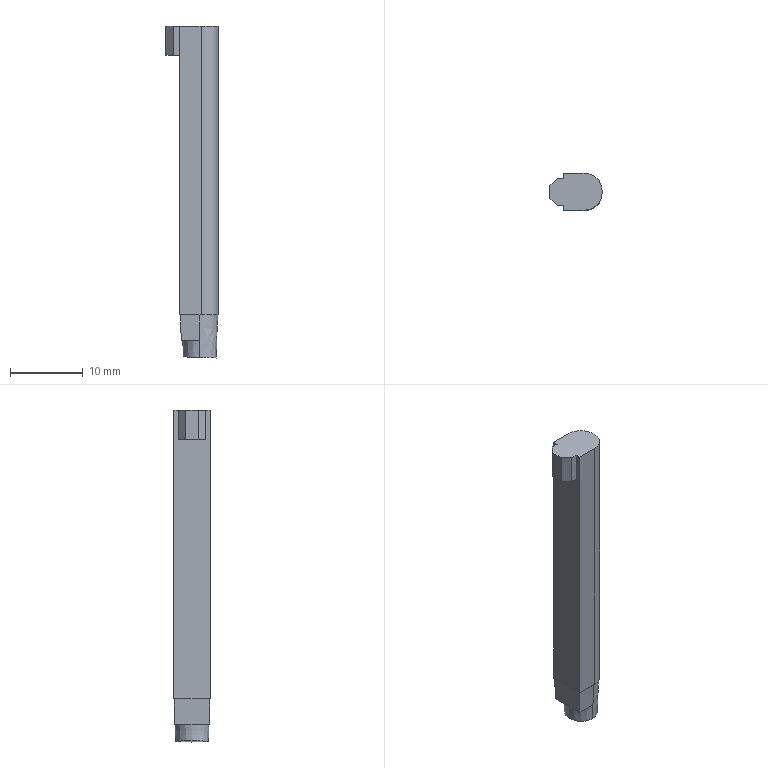Part | Creo | 1 solid | 21 faces | box 7.184 x 5.033 x 45.741 mm | volume 1104 mm3 | plane 17 | cylinder 2 | spline 2 | commonest cylinder face diameters 4.7 x2
STEP:
#1=CARTESIAN_POINT('',(0.,0.,0.));
#2=DIRECTION('',(0.,0.,1.));
#3=DIRECTION('',(1.,0.,0.));
#4=AXIS2_PLACEMENT_3D('',#1,#2,#3);
#5=CARTESIAN_POINT('',(-43.549,78.476,85.91));
#6=VERTEX_POINT('',#5);
#7=CARTESIAN_POINT('',(-43.549,78.476,46.111));
#8=VERTEX_POINT('',#7);
#9=CARTESIAN_POINT('',(-43.549,78.476,85.91));
#10=DIRECTION('',(0.,0.,-1.));
#11=VECTOR('',#10,39.799);
#12=LINE('',#9,#11);
#13=EDGE_CURVE('',#6,#8,#12,.T.);
#14=ORIENTED_EDGE('',*,*,#13,.F.);
#15=CARTESIAN_POINT('',(-40.614,78.476,85.91));
#16=VERTEX_POINT('',#15);
#17=CARTESIAN_POINT('',(-43.549,78.476,85.91));
#18=DIRECTION('',(1.,0.,0.));
#19=VECTOR('',#18,2.934);
#20=LINE('',#17,#19);
#21=EDGE_CURVE('',#6,#16,#20,.T.);
#22=ORIENTED_EDGE('',*,*,#21,.T.);
#23=CARTESIAN_POINT('',(-40.614,78.476,46.111));
#24=VERTEX_POINT('',#23);
#25=CARTESIAN_POINT('',(-40.614,78.476,85.91));
#26=DIRECTION('',(0.,0.,-1.));
#27=VECTOR('',#26,39.799);
#28=LINE('',#25,#27);
#29=EDGE_CURVE('',#16,#24,#28,.T.);
#30=ORIENTED_EDGE('',*,*,#29,.T.);
#31=CARTESIAN_POINT('',(-40.614,78.476,46.111));
#32=DIRECTION('',(-1.,0.,0.));
#33=VECTOR('',#32,2.934);
#34=LINE('',#31,#33);
#35=EDGE_CURVE('',#24,#8,#34,.T.);
#36=ORIENTED_EDGE('',*,*,#35,.T.);
#37=EDGE_LOOP('',(#14,#22,#30,#36));
#38=FACE_OUTER_BOUND('',#37,.F.);
#39=CARTESIAN_POINT('',(-40.806,78.476,6.695));
#40=DIRECTION('',(0.,-1.,0.));
#41=DIRECTION('',(0.,0.,-1.));
#42=AXIS2_PLACEMENT_3D('',#39,#40,#41);
#43=PLANE('',#42);
#44=ADVANCED_FACE('',(#38),#43,.T.);
#45=CARTESIAN_POINT('',(-43.549,83.509,85.91));
#46=VERTEX_POINT('',#45);
#47=CARTESIAN_POINT('',(-43.549,83.509,46.111));
#48=VERTEX_POINT('',#47);
#49=CARTESIAN_POINT('',(-43.549,83.509,85.91));
#50=DIRECTION('',(0.,0.,-1.));
#51=VECTOR('',#50,39.799);
#52=LINE('',#49,#51);
#53=EDGE_CURVE('',#46,#48,#52,.T.);
#54=ORIENTED_EDGE('',*,*,#53,.F.);
#55=CARTESIAN_POINT('',(-43.549,82.859,85.91));
#56=VERTEX_POINT('',#55);
#57=CARTESIAN_POINT('',(-43.549,83.509,85.91));
#58=DIRECTION('',(0.,-1.,0.));
#59=VECTOR('',#58,0.65);
#60=LINE('',#57,#59);
#61=EDGE_CURVE('',#46,#56,#60,.T.);
#62=ORIENTED_EDGE('',*,*,#61,.T.);
#63=CARTESIAN_POINT('',(-43.549,82.859,81.91));
#64=VERTEX_POINT('',#63);
#65=CARTESIAN_POINT('',(-43.549,82.859,81.91));
#66=DIRECTION('',(0.,0.,1.));
#67=VECTOR('',#66,4.);
#68=LINE('',#65,#67);
#69=EDGE_CURVE('',#64,#56,#68,.T.);
#70=ORIENTED_EDGE('',*,*,#69,.F.);
#71=CARTESIAN_POINT('',(-43.549,79.126,81.91));
#72=VERTEX_POINT('',#71);
#73=CARTESIAN_POINT('',(-43.549,79.126,81.91));
#74=DIRECTION('',(0.,1.,0.));
#75=VECTOR('',#74,3.733);
#76=LINE('',#73,#75);
#77=EDGE_CURVE('',#72,#64,#76,.T.);
#78=ORIENTED_EDGE('',*,*,#77,.F.);
#79=CARTESIAN_POINT('',(-43.549,79.126,85.91));
#80=VERTEX_POINT('',#79);
#81=CARTESIAN_POINT('',(-43.549,79.126,85.91));
#82=DIRECTION('',(0.,0.,-1.));
#83=VECTOR('',#82,4.);
#84=LINE('',#81,#83);
#85=EDGE_CURVE('',#80,#72,#84,.T.);
#86=ORIENTED_EDGE('',*,*,#85,.F.);
#87=CARTESIAN_POINT('',(-43.549,79.126,85.91));
#88=DIRECTION('',(0.,-1.,0.));
#89=VECTOR('',#88,0.65);
#90=LINE('',#87,#89);
#91=EDGE_CURVE('',#80,#6,#90,.T.);
#92=ORIENTED_EDGE('',*,*,#91,.T.);
#93=ORIENTED_EDGE('',*,*,#13,.T.);
#94=CARTESIAN_POINT('',(-43.549,78.476,46.111));
#95=DIRECTION('',(0.,1.,0.));
#96=VECTOR('',#95,5.033);
#97=LINE('',#94,#96);
#98=EDGE_CURVE('',#8,#48,#97,.T.);
#99=ORIENTED_EDGE('',*,*,#98,.T.);
#100=EDGE_LOOP('',(#54,#62,#70,#78,#86,#92,#93,#99));
#101=FACE_OUTER_BOUND('',#100,.F.);
#102=CARTESIAN_POINT('',(-43.549,80.993,6.695));
#103=DIRECTION('',(-1.,0.,0.));
#104=DIRECTION('',(0.,0.,1.));
#105=AXIS2_PLACEMENT_3D('',#102,#103,#104);
#106=PLANE('',#105);
#107=ADVANCED_FACE('',(#101),#106,.T.);
#108=CARTESIAN_POINT('',(-40.614,83.509,46.111));
#109=VERTEX_POINT('',#108);
#110=CARTESIAN_POINT('',(-40.614,83.509,85.91));
#111=VERTEX_POINT('',#110);
#112=CARTESIAN_POINT('',(-40.614,83.509,46.111));
#113=DIRECTION('',(0.,0.,1.));
#114=VECTOR('',#113,39.799);
#115=LINE('',#112,#114);
#116=EDGE_CURVE('',#109,#111,#115,.T.);
#117=ORIENTED_EDGE('',*,*,#116,.T.);
#118=CARTESIAN_POINT('',(-40.614,83.509,85.91));
#119=DIRECTION('',(-1.,0.,0.));
#120=VECTOR('',#119,2.934);
#121=LINE('',#118,#120);
#122=EDGE_CURVE('',#111,#46,#121,.T.);
#123=ORIENTED_EDGE('',*,*,#122,.T.);
#124=ORIENTED_EDGE('',*,*,#53,.T.);
#125=CARTESIAN_POINT('',(-43.549,83.509,46.111));
#126=DIRECTION('',(1.,0.,0.));
#127=VECTOR('',#126,2.934);
#128=LINE('',#125,#127);
#129=EDGE_CURVE('',#48,#109,#128,.T.);
#130=ORIENTED_EDGE('',*,*,#129,.T.);
#131=EDGE_LOOP('',(#117,#123,#124,#130));
#132=FACE_OUTER_BOUND('',#131,.F.);
#133=CARTESIAN_POINT('',(-40.806,83.509,6.695));
#134=DIRECTION('',(0.,1.,0.));
#135=DIRECTION('',(0.,0.,1.));
#136=AXIS2_PLACEMENT_3D('',#133,#134,#135);
#137=PLANE('',#136);
#138=ADVANCED_FACE('',(#132),#137,.T.);
#139=CARTESIAN_POINT('',(-38.264,81.159,85.91));
#140=VERTEX_POINT('',#139);
#141=CARTESIAN_POINT('',(-38.264,81.159,46.111));
#142=VERTEX_POINT('',#141);
#143=CARTESIAN_POINT('',(-38.264,81.159,85.91));
#144=DIRECTION('',(0.,0.,-1.));
#145=VECTOR('',#144,39.799);
#146=LINE('',#143,#145);
#147=EDGE_CURVE('',#140,#142,#146,.T.);
#148=ORIENTED_EDGE('',*,*,#147,.F.);
#149=CARTESIAN_POINT('',(-40.614,81.159,85.91));
#150=DIRECTION('',(0.,0.,1.));
#151=DIRECTION('',(1.,0.,0.));
#152=AXIS2_PLACEMENT_3D('',#149,#150,#151);
#153=CIRCLE('',#152,2.35);
#154=EDGE_CURVE('',#140,#111,#153,.T.);
#155=ORIENTED_EDGE('',*,*,#154,.T.);
#156=ORIENTED_EDGE('',*,*,#116,.F.);
#157=CARTESIAN_POINT('',(-40.614,81.159,46.111));
#158=DIRECTION('',(0.,0.,-1.));
#159=DIRECTION('',(0.,1.,0.));
#160=AXIS2_PLACEMENT_3D('',#157,#158,#159);
#161=CIRCLE('',#160,2.35);
#162=EDGE_CURVE('',#109,#142,#161,.T.);
#163=ORIENTED_EDGE('',*,*,#162,.T.);
#164=EDGE_LOOP('',(#148,#155,#156,#163));
#165=FACE_OUTER_BOUND('',#164,.F.);
#166=CARTESIAN_POINT('',(-40.614,81.159,6.695));
#167=DIRECTION('',(0.,0.,1.));
#168=DIRECTION('',(1.,0.,0.));
#169=AXIS2_PLACEMENT_3D('',#166,#167,#168);
#170=CYLINDRICAL_SURFACE('',#169,2.35);
#171=ADVANCED_FACE('',(#165),#170,.T.);
#172=CARTESIAN_POINT('',(-38.264,80.826,46.111));
#173=VERTEX_POINT('',#172);
#174=CARTESIAN_POINT('',(-38.264,80.826,85.91));
#175=VERTEX_POINT('',#174);
#176=CARTESIAN_POINT('',(-38.264,80.826,46.111));
#177=DIRECTION('',(0.,0.,1.));
#178=VECTOR('',#177,39.799);
#179=LINE('',#176,#178);
#180=EDGE_CURVE('',#173,#175,#179,.T.);
#181=ORIENTED_EDGE('',*,*,#180,.T.);
#182=CARTESIAN_POINT('',(-38.264,80.826,85.91));
#183=DIRECTION('',(0.,1.,0.));
#184=VECTOR('',#183,0.333);
#185=LINE('',#182,#184);
#186=EDGE_CURVE('',#175,#140,#185,.T.);
#187=ORIENTED_EDGE('',*,*,#186,.T.);
#188=ORIENTED_EDGE('',*,*,#147,.T.);
#189=CARTESIAN_POINT('',(-38.264,81.159,46.111));
#190=DIRECTION('',(0.,-1.,0.));
#191=VECTOR('',#190,0.333);
#192=LINE('',#189,#191);
#193=EDGE_CURVE('',#142,#173,#192,.T.);
#194=ORIENTED_EDGE('',*,*,#193,.T.);
#195=EDGE_LOOP('',(#181,#187,#188,#194));
#196=FACE_OUTER_BOUND('',#195,.F.);
#197=CARTESIAN_POINT('',(-38.264,80.993,6.695));
#198=DIRECTION('',(1.,0.,0.));
#199=DIRECTION('',(0.,0.,-1.));
#200=AXIS2_PLACEMENT_3D('',#197,#198,#199);
#201=PLANE('',#200);
#202=ADVANCED_FACE('',(#196),#201,.T.);
#203=ORIENTED_EDGE('',*,*,#29,.F.);
#204=CARTESIAN_POINT('',(-40.614,80.826,85.91));
#205=DIRECTION('',(0.,0.,1.));
#206=DIRECTION('',(0.,-1.,0.));
#207=AXIS2_PLACEMENT_3D('',#204,#205,#206);
#208=CIRCLE('',#207,2.35);
#209=EDGE_CURVE('',#16,#175,#208,.T.);
#210=ORIENTED_EDGE('',*,*,#209,.T.);
#211=ORIENTED_EDGE('',*,*,#180,.F.);
#212=CARTESIAN_POINT('',(-40.614,80.826,46.111));
#213=DIRECTION('',(0.,0.,-1.));
#214=DIRECTION('',(1.,0.,0.));
#215=AXIS2_PLACEMENT_3D('',#212,#213,#214);
#216=CIRCLE('',#215,2.35);
#217=EDGE_CURVE('',#173,#24,#216,.T.);
#218=ORIENTED_EDGE('',*,*,#217,.T.);
#219=EDGE_LOOP('',(#203,#210,#211,#218));
#220=FACE_OUTER_BOUND('',#219,.F.);
#221=CARTESIAN_POINT('',(-40.614,80.826,6.695));
#222=DIRECTION('',(0.,0.,1.));
#223=DIRECTION('',(1.,0.,0.));
#224=AXIS2_PLACEMENT_3D('',#221,#222,#223);
#225=CYLINDRICAL_SURFACE('',#224,2.35);
#226=ADVANCED_FACE('',(#220),#225,.T.);
#227=CARTESIAN_POINT('',(-45.449,81.859,85.91));
#228=VERTEX_POINT('',#227);
#229=CARTESIAN_POINT('',(-45.449,80.126,85.91));
#230=VERTEX_POINT('',#229);
#231=CARTESIAN_POINT('',(-45.449,81.859,85.91));
#232=DIRECTION('',(0.,-1.,0.));
#233=VECTOR('',#232,1.733);
#234=LINE('',#231,#233);
#235=EDGE_CURVE('',#228,#230,#234,.T.);
#236=ORIENTED_EDGE('',*,*,#235,.F.);
#237=CARTESIAN_POINT('',(-44.449,82.859,85.91));
#238=VERTEX_POINT('',#237);
#239=CARTESIAN_POINT('',(-44.449,82.859,85.91));
#240=DIRECTION('',(-0.7071,-0.7071,0.));
#241=VECTOR('',#240,1.414);
#242=LINE('',#239,#241);
#243=EDGE_CURVE('',#238,#228,#242,.T.);
#244=ORIENTED_EDGE('',*,*,#243,.F.);
#245=CARTESIAN_POINT('',(-43.549,82.859,85.91));
#246=DIRECTION('',(-1.,0.,0.));
#247=VECTOR('',#246,0.9);
#248=LINE('',#245,#247);
#249=EDGE_CURVE('',#56,#238,#248,.T.);
#250=ORIENTED_EDGE('',*,*,#249,.F.);
#251=ORIENTED_EDGE('',*,*,#61,.F.);
#252=ORIENTED_EDGE('',*,*,#122,.F.);
#253=ORIENTED_EDGE('',*,*,#154,.F.);
#254=ORIENTED_EDGE('',*,*,#186,.F.);
#255=ORIENTED_EDGE('',*,*,#209,.F.);
#256=ORIENTED_EDGE('',*,*,#21,.F.);
#257=ORIENTED_EDGE('',*,*,#91,.F.);
#258=CARTESIAN_POINT('',(-44.449,79.126,85.91));
#259=VERTEX_POINT('',#258);
#260=CARTESIAN_POINT('',(-44.449,79.126,85.91));
#261=DIRECTION('',(1.,0.,0.));
#262=VECTOR('',#261,0.9);
#263=LINE('',#260,#262);
#264=EDGE_CURVE('',#259,#80,#263,.T.);
#265=ORIENTED_EDGE('',*,*,#264,.F.);
#266=CARTESIAN_POINT('',(-45.449,80.126,85.91));
#267=DIRECTION('',(0.7071,-0.7071,0.));
#268=VECTOR('',#267,1.414);
#269=LINE('',#266,#268);
#270=EDGE_CURVE('',#230,#259,#269,.T.);
#271=ORIENTED_EDGE('',*,*,#270,.F.);
#272=EDGE_LOOP('',(#236,#244,#250,#251,#252,#253,#254,#255,#256,#257,#265,#271));
#273=FACE_OUTER_BOUND('',#272,.F.);
#274=CARTESIAN_POINT('',(62.144,-0.4125,85.91));
#275=DIRECTION('',(0.,0.,1.));
#276=DIRECTION('',(0.,1.,0.));
#277=AXIS2_PLACEMENT_3D('',#274,#275,#276);
#278=PLANE('',#277);
#279=ADVANCED_FACE('',(#273),#278,.T.);
#280=CARTESIAN_POINT('',(-45.449,80.126,81.91));
#281=VERTEX_POINT('',#280);
#282=CARTESIAN_POINT('',(-45.449,81.859,81.91));
#283=VERTEX_POINT('',#282);
#284=CARTESIAN_POINT('',(-45.449,80.126,81.91));
#285=DIRECTION('',(0.,1.,0.));
#286=VECTOR('',#285,1.733);
#287=LINE('',#284,#286);
#288=EDGE_CURVE('',#281,#283,#287,.T.);
#289=ORIENTED_EDGE('',*,*,#288,.T.);
#290=CARTESIAN_POINT('',(-45.449,81.859,81.91));
#291=DIRECTION('',(0.,0.,1.));
#292=VECTOR('',#291,4.);
#293=LINE('',#290,#292);
#294=EDGE_CURVE('',#283,#228,#293,.T.);
#295=ORIENTED_EDGE('',*,*,#294,.T.);
#296=ORIENTED_EDGE('',*,*,#235,.T.);
#297=CARTESIAN_POINT('',(-45.449,80.126,85.91));
#298=DIRECTION('',(0.,0.,-1.));
#299=VECTOR('',#298,4.);
#300=LINE('',#297,#299);
#301=EDGE_CURVE('',#230,#281,#300,.T.);
#302=ORIENTED_EDGE('',*,*,#301,.T.);
#303=EDGE_LOOP('',(#289,#295,#296,#302));
#304=FACE_OUTER_BOUND('',#303,.F.);
#305=CARTESIAN_POINT('',(-45.449,80.993,81.91));
#306=DIRECTION('',(-1.,0.,0.));
#307=DIRECTION('',(0.,0.,1.));
#308=AXIS2_PLACEMENT_3D('',#305,#306,#307);
#309=PLANE('',#308);
#310=ADVANCED_FACE('',(#304),#309,.T.);
#311=CARTESIAN_POINT('',(-44.449,79.126,81.91));
#312=VERTEX_POINT('',#311);
#313=CARTESIAN_POINT('',(-43.549,79.126,81.91));
#314=DIRECTION('',(-1.,0.,0.));
#315=VECTOR('',#314,0.9);
#316=LINE('',#313,#315);
#317=EDGE_CURVE('',#72,#312,#316,.T.);
#318=ORIENTED_EDGE('',*,*,#317,.F.);
#319=ORIENTED_EDGE('',*,*,#77,.T.);
#320=CARTESIAN_POINT('',(-44.449,82.859,81.91));
#321=VERTEX_POINT('',#320);
#322=CARTESIAN_POINT('',(-44.449,82.859,81.91));
#323=DIRECTION('',(1.,0.,0.));
#324=VECTOR('',#323,0.9);
#325=LINE('',#322,#324);
#326=EDGE_CURVE('',#321,#64,#325,.T.);
#327=ORIENTED_EDGE('',*,*,#326,.F.);
#328=CARTESIAN_POINT('',(-45.449,81.859,81.91));
#329=DIRECTION('',(0.7071,0.7071,0.));
#330=VECTOR('',#329,1.414);
#331=LINE('',#328,#330);
#332=EDGE_CURVE('',#283,#321,#331,.T.);
#333=ORIENTED_EDGE('',*,*,#332,.F.);
#334=ORIENTED_EDGE('',*,*,#288,.F.);
#335=CARTESIAN_POINT('',(-44.449,79.126,81.91));
#336=DIRECTION('',(-0.7071,0.7071,0.));
#337=VECTOR('',#336,1.414);
#338=LINE('',#335,#337);
#339=EDGE_CURVE('',#312,#281,#338,.T.);
#340=ORIENTED_EDGE('',*,*,#339,.F.);
#341=EDGE_LOOP('',(#318,#319,#327,#333,#334,#340));
#342=FACE_OUTER_BOUND('',#341,.F.);
#343=CARTESIAN_POINT('',(-43.899,80.993,81.91));
#344=DIRECTION('',(0.,0.,-1.));
#345=DIRECTION('',(-1.,0.,0.));
#346=AXIS2_PLACEMENT_3D('',#343,#344,#345);
#347=PLANE('',#346);
#348=ADVANCED_FACE('',(#342),#347,.T.);
#349=ORIENTED_EDGE('',*,*,#264,.T.);
#350=ORIENTED_EDGE('',*,*,#85,.T.);
#351=ORIENTED_EDGE('',*,*,#317,.T.);
#352=CARTESIAN_POINT('',(-44.449,79.126,81.91));
#353=DIRECTION('',(0.,0.,1.));
#354=VECTOR('',#353,4.);
#355=LINE('',#352,#354);
#356=EDGE_CURVE('',#312,#259,#355,.T.);
#357=ORIENTED_EDGE('',*,*,#356,.T.);
#358=EDGE_LOOP('',(#349,#350,#351,#357));
#359=FACE_OUTER_BOUND('',#358,.F.);
#360=CARTESIAN_POINT('',(-43.899,79.126,81.91));
#361=DIRECTION('',(0.,-1.,0.));
#362=DIRECTION('',(0.,0.,-1.));
#363=AXIS2_PLACEMENT_3D('',#360,#361,#362);
#364=PLANE('',#363);
#365=ADVANCED_FACE('',(#359),#364,.T.);
#366=ORIENTED_EDGE('',*,*,#339,.T.);
#367=ORIENTED_EDGE('',*,*,#301,.F.);
#368=ORIENTED_EDGE('',*,*,#270,.T.);
#369=ORIENTED_EDGE('',*,*,#356,.F.);
#370=EDGE_LOOP('',(#366,#367,#368,#369));
#371=FACE_OUTER_BOUND('',#370,.F.);
#372=CARTESIAN_POINT('',(-45.449,80.126,81.91));
#373=DIRECTION('',(0.7071,0.7071,0.));
#374=DIRECTION('',(0.,0.,1.));
#375=AXIS2_PLACEMENT_3D('',#372,#373,#374);
#376=PLANE('',#375);
#377=ADVANCED_FACE('',(#371),#376,.F.);
#378=ORIENTED_EDGE('',*,*,#326,.T.);
#379=ORIENTED_EDGE('',*,*,#69,.T.);
#380=ORIENTED_EDGE('',*,*,#249,.T.);
#381=CARTESIAN_POINT('',(-44.449,82.859,85.91));
#382=DIRECTION('',(0.,0.,-1.));
#383=VECTOR('',#382,4.);
#384=LINE('',#381,#383);
#385=EDGE_CURVE('',#238,#321,#384,.T.);
#386=ORIENTED_EDGE('',*,*,#385,.T.);
#387=EDGE_LOOP('',(#378,#379,#380,#386));
#388=FACE_OUTER_BOUND('',#387,.F.);
#389=CARTESIAN_POINT('',(-43.899,82.859,81.91));
#390=DIRECTION('',(0.,1.,0.));
#391=DIRECTION('',(0.,0.,1.));
#392=AXIS2_PLACEMENT_3D('',#389,#390,#391);
#393=PLANE('',#392);
#394=ADVANCED_FACE('',(#388),#393,.T.);
#395=ORIENTED_EDGE('',*,*,#332,.T.);
#396=ORIENTED_EDGE('',*,*,#385,.F.);
#397=ORIENTED_EDGE('',*,*,#243,.T.);
#398=ORIENTED_EDGE('',*,*,#294,.F.);
#399=EDGE_LOOP('',(#395,#396,#397,#398));
#400=FACE_OUTER_BOUND('',#399,.F.);
#401=CARTESIAN_POINT('',(-44.449,82.859,81.91));
#402=DIRECTION('',(0.7071,-0.7071,0.));
#403=DIRECTION('',(0.,0.,1.));
#404=AXIS2_PLACEMENT_3D('',#401,#402,#403);
#405=PLANE('',#404);
#406=ADVANCED_FACE('',(#400),#405,.F.);
#407=ORIENTED_EDGE('',*,*,#217,.F.);
#408=ORIENTED_EDGE('',*,*,#193,.F.);
#409=ORIENTED_EDGE('',*,*,#162,.F.);
#410=ORIENTED_EDGE('',*,*,#129,.F.);
#411=ORIENTED_EDGE('',*,*,#98,.F.);
#412=ORIENTED_EDGE('',*,*,#35,.F.);
#413=EDGE_LOOP('',(#407,#408,#409,#410,#411,#412));
#414=FACE_OUTER_BOUND('',#413,.F.);
#415=CARTESIAN_POINT('',(-38.311,80.993,46.111));
#416=VERTEX_POINT('',#415);
#417=CARTESIAN_POINT('',(-40.781,78.524,46.111));
#418=VERTEX_POINT('',#417);
#419=CARTESIAN_POINT('',(-38.311,80.834,46.111));
#420=CARTESIAN_POINT('',(-38.341,80.522,46.111));
#421=CARTESIAN_POINT('',(-38.481,80.056,46.111));
#422=CARTESIAN_POINT('',(-38.709,79.62,46.111));
#423=CARTESIAN_POINT('',(-39.022,79.234,46.111));
#424=CARTESIAN_POINT('',(-39.408,78.921,46.111));
#425=CARTESIAN_POINT('',(-39.844,78.693,46.111));
#426=CARTESIAN_POINT('',(-40.311,78.554,46.111));
#427=CARTESIAN_POINT('',(-40.623,78.524,46.111));
#428=CARTESIAN_POINT('',(-40.781,78.524,46.111));
#429=B_SPLINE_CURVE_WITH_KNOTS('',3,(#415,#419,#420,#421,#422,#423,#424,#425,#426,#427,#428),.UNSPECIFIED.,.F.,.F.,(4,1,1,1,1,1,1,1,4),(0.,0.125,0.25,0.375,0.5,0.625,0.75,0.875,1.),.UNSPECIFIED.);
#430=EDGE_CURVE('',#416,#418,#429,.T.);
#431=ORIENTED_EDGE('',*,*,#430,.T.);
#432=CARTESIAN_POINT('',(-43.46,78.525,46.111));
#433=VERTEX_POINT('',#432);
#434=CARTESIAN_POINT('',(-43.46,78.525,46.111));
#435=DIRECTION('',(1.,-0.0005637,0.000000177));
#436=VECTOR('',#435,2.679);
#437=LINE('',#434,#436);
#438=EDGE_CURVE('',#433,#418,#437,.T.);
#439=ORIENTED_EDGE('',*,*,#438,.F.);
#440=CARTESIAN_POINT('',(-43.46,83.46,46.111));
#441=VERTEX_POINT('',#440);
#442=CARTESIAN_POINT('',(-43.46,83.46,46.111));
#443=DIRECTION('',(0.,-1.,0.));
#444=VECTOR('',#443,4.935);
#445=LINE('',#442,#444);
#446=EDGE_CURVE('',#441,#433,#445,.T.);
#447=ORIENTED_EDGE('',*,*,#446,.F.);
#448=CARTESIAN_POINT('',(-40.781,83.461,46.111));
#449=VERTEX_POINT('',#448);
#450=CARTESIAN_POINT('',(-40.781,83.461,46.111));
#451=DIRECTION('',(-1.,-0.0005749,0.000001935));
#452=VECTOR('',#451,2.679);
#453=LINE('',#450,#452);
#454=EDGE_CURVE('',#449,#441,#453,.T.);
#455=ORIENTED_EDGE('',*,*,#454,.F.);
#456=CARTESIAN_POINT('',(-40.781,83.461,46.111));
#457=CARTESIAN_POINT('',(-40.623,83.461,46.111));
#458=CARTESIAN_POINT('',(-40.311,83.431,46.111));
#459=CARTESIAN_POINT('',(-39.844,83.292,46.111));
#460=CARTESIAN_POINT('',(-39.408,83.063,46.111));
#461=CARTESIAN_POINT('',(-39.022,82.751,46.111));
#462=CARTESIAN_POINT('',(-38.709,82.365,46.111));
#463=CARTESIAN_POINT('',(-38.481,81.929,46.111));
#464=CARTESIAN_POINT('',(-38.341,81.463,46.111));
#465=CARTESIAN_POINT('',(-38.311,81.151,46.111));
#466=CARTESIAN_POINT('',(-38.311,80.993,46.111));
#467=B_SPLINE_CURVE_WITH_KNOTS('',3,(#456,#457,#458,#459,#460,#461,#462,#463,#464,#465,#466),.UNSPECIFIED.,.F.,.F.,(4,1,1,1,1,1,1,1,4),(0.,0.125,0.25,0.375,0.5,0.625,0.75,0.875,1.),.UNSPECIFIED.);
#468=EDGE_CURVE('',#449,#416,#467,.T.);
#469=ORIENTED_EDGE('',*,*,#468,.T.);
#470=EDGE_LOOP('',(#431,#439,#447,#455,#469));
#471=FACE_BOUND('',#470,.F.);
#472=CARTESIAN_POINT('',(-45.303,-88.35,46.111));
#473=DIRECTION('',(0.,0.,1.));
#474=DIRECTION('',(-1.,0.,0.));
#475=AXIS2_PLACEMENT_3D('',#472,#473,#474);
#476=PLANE('',#475);
#477=ADVANCED_FACE('',(#414,#471),#476,.F.);
#478=CARTESIAN_POINT('',(-40.78,78.646,42.593));
#479=VERTEX_POINT('',#478);
#480=CARTESIAN_POINT('',(-40.781,78.524,46.111));
#481=DIRECTION('',(0.0003501,0.03487,-0.9994));
#482=VECTOR('',#481,3.52);
#483=LINE('',#480,#482);
#484=EDGE_CURVE('',#418,#479,#483,.T.);
#485=ORIENTED_EDGE('',*,*,#484,.F.);
#486=ORIENTED_EDGE('',*,*,#430,.F.);
#487=ORIENTED_EDGE('',*,*,#468,.F.);
#488=CARTESIAN_POINT('',(-40.78,83.339,42.593));
#489=VERTEX_POINT('',#488);
#490=CARTESIAN_POINT('',(-40.781,83.461,46.111));
#491=DIRECTION('',(0.0003494,-0.03488,-0.9994));
#492=VECTOR('',#491,3.52);
#493=LINE('',#490,#492);
#494=EDGE_CURVE('',#449,#489,#493,.T.);
#495=ORIENTED_EDGE('',*,*,#494,.T.);
#496=CARTESIAN_POINT('',(-40.781,83.257,40.248));
#497=VERTEX_POINT('',#496);
#498=CARTESIAN_POINT('',(-40.781,83.257,40.248));
#499=DIRECTION('',(0.0004719,0.0349,0.9994));
#500=VECTOR('',#499,2.347);
#501=LINE('',#498,#500);
#502=EDGE_CURVE('',#497,#489,#501,.T.);
#503=ORIENTED_EDGE('',*,*,#502,.F.);
#504=CARTESIAN_POINT('',(-38.518,80.993,40.169));
#505=VERTEX_POINT('',#504);
#506=CARTESIAN_POINT('',(-40.607,83.257,40.242));
#507=CARTESIAN_POINT('',(-40.271,83.218,40.23));
#508=CARTESIAN_POINT('',(-39.788,83.048,40.213));
#509=CARTESIAN_POINT('',(-39.357,82.777,40.198));
#510=CARTESIAN_POINT('',(-38.998,82.417,40.185));
#511=CARTESIAN_POINT('',(-38.726,81.986,40.176));
#512=CARTESIAN_POINT('',(-38.557,81.502,40.17));
#513=CARTESIAN_POINT('',(-38.518,81.166,40.169));
#514=B_SPLINE_CURVE_WITH_KNOTS('',3,(#496,#506,#507,#508,#509,#510,#511,#512,#513,#504),.UNSPECIFIED.,.F.,.F.,(4,1,1,1,1,1,1,4),(0.,0.1429,0.2857,0.4286,0.5714,0.7143,0.8571,1.),.UNSPECIFIED.);
#515=EDGE_CURVE('',#497,#505,#514,.T.);
#516=ORIENTED_EDGE('',*,*,#515,.T.);
#517=CARTESIAN_POINT('',(-40.781,78.728,40.248));
#518=VERTEX_POINT('',#517);
#519=CARTESIAN_POINT('',(-38.518,80.993,40.169));
#520=CARTESIAN_POINT('',(-38.518,80.819,40.169));
#521=CARTESIAN_POINT('',(-38.557,80.483,40.17));
#522=CARTESIAN_POINT('',(-38.726,79.999,40.176));
#523=CARTESIAN_POINT('',(-38.998,79.568,40.185));
#524=CARTESIAN_POINT('',(-39.357,79.208,40.198));
#525=CARTESIAN_POINT('',(-39.788,78.937,40.213));
#526=CARTESIAN_POINT('',(-40.271,78.767,40.23));
#527=CARTESIAN_POINT('',(-40.607,78.728,40.242));
#528=B_SPLINE_CURVE_WITH_KNOTS('',3,(#519,#520,#521,#522,#523,#524,#525,#526,#527,#517),.UNSPECIFIED.,.F.,.F.,(4,1,1,1,1,1,1,4),(0.,0.1429,0.2857,0.4286,0.5714,0.7143,0.8571,1.),.UNSPECIFIED.);
#529=EDGE_CURVE('',#505,#518,#528,.T.);
#530=ORIENTED_EDGE('',*,*,#529,.T.);
#531=CARTESIAN_POINT('',(-40.78,78.646,42.593));
#532=DIRECTION('',(-0.0004715,0.03491,-0.9994));
#533=VECTOR('',#532,2.347);
#534=LINE('',#531,#533);
#535=EDGE_CURVE('',#479,#518,#534,.T.);
#536=ORIENTED_EDGE('',*,*,#535,.F.);
#537=EDGE_LOOP('',(#485,#486,#487,#495,#503,#516,#530,#536));
#538=FACE_OUTER_BOUND('',#537,.F.);
#539=CARTESIAN_POINT('',(-40.936,83.463,46.314));
#540=CARTESIAN_POINT('',(-40.932,83.392,44.254));
#541=CARTESIAN_POINT('',(-40.927,83.32,42.194));
#542=CARTESIAN_POINT('',(-40.923,83.248,40.134));
#543=CARTESIAN_POINT('',(-40.885,83.467,46.312));
#544=CARTESIAN_POINT('',(-40.881,83.395,44.252));
#545=CARTESIAN_POINT('',(-40.878,83.323,42.192));
#546=CARTESIAN_POINT('',(-40.875,83.251,40.132));
#547=CARTESIAN_POINT('',(-40.185,83.489,46.29));
#548=CARTESIAN_POINT('',(-40.202,83.417,44.23));
#549=CARTESIAN_POINT('',(-40.219,83.344,42.17));
#550=CARTESIAN_POINT('',(-40.237,83.272,40.11));
#551=CARTESIAN_POINT('',(-38.843,82.933,46.247));
#552=CARTESIAN_POINT('',(-38.899,82.876,44.187));
#553=CARTESIAN_POINT('',(-38.955,82.82,42.127));
#554=CARTESIAN_POINT('',(-39.012,82.764,40.067));
#555=CARTESIAN_POINT('',(-38.038,80.992,46.221));
#556=CARTESIAN_POINT('',(-38.118,80.992,44.161));
#557=CARTESIAN_POINT('',(-38.198,80.992,42.101));
#558=CARTESIAN_POINT('',(-38.278,80.992,40.041));
#559=CARTESIAN_POINT('',(-38.843,79.052,46.247));
#560=CARTESIAN_POINT('',(-38.899,79.109,44.187));
#561=CARTESIAN_POINT('',(-38.955,79.165,42.127));
#562=CARTESIAN_POINT('',(-39.012,79.221,40.067));
#563=CARTESIAN_POINT('',(-40.185,78.496,46.29));
#564=CARTESIAN_POINT('',(-40.202,78.568,44.23));
#565=CARTESIAN_POINT('',(-40.219,78.641,42.17));
#566=CARTESIAN_POINT('',(-40.237,78.713,40.11));
#567=CARTESIAN_POINT('',(-40.885,78.518,46.312));
#568=CARTESIAN_POINT('',(-40.881,78.59,44.252));
#569=CARTESIAN_POINT('',(-40.878,78.662,42.192));
#570=CARTESIAN_POINT('',(-40.875,78.734,40.132));
#571=CARTESIAN_POINT('',(-40.936,78.522,46.314));
#572=CARTESIAN_POINT('',(-40.932,78.593,44.254));
#573=CARTESIAN_POINT('',(-40.927,78.665,42.194));
#574=CARTESIAN_POINT('',(-40.923,78.737,40.134));
#575=B_SPLINE_SURFACE_WITH_KNOTS('',3,3,((#539,#540,#541,#542),(#543,#544,#545,#546),(#547,#548,#549,#550),(#551,#552,#553,#554),(#555,#556,#557,#558),(#559,#560,#561,#562),(#563,#564,#565,#566),(#567,#568,#569,#570),(#571,#572,#573,#574)),.UNSPECIFIED.,.F.,.F.,.F.,(4,1,1,1,1,1,4),(4,4),(-0.02,0.,0.25,0.5,0.75,1.,1.02),(0.1461,0.9903),.UNSPECIFIED.);
#576=ADVANCED_FACE('',(#538),#575,.T.);
#577=CARTESIAN_POINT('',(-43.337,78.648,42.593));
#578=VERTEX_POINT('',#577);
#579=CARTESIAN_POINT('',(-43.46,78.525,46.111));
#580=DIRECTION('',(0.03488,0.03486,-0.9988));
#581=VECTOR('',#580,3.522);
#582=LINE('',#579,#581);
#583=EDGE_CURVE('',#433,#578,#582,.T.);
#584=ORIENTED_EDGE('',*,*,#583,.F.);
#585=ORIENTED_EDGE('',*,*,#438,.T.);
#586=ORIENTED_EDGE('',*,*,#484,.T.);
#587=CARTESIAN_POINT('',(-43.337,78.648,42.593));
#588=DIRECTION('',(1.,-0.0006061,-0.000001412));
#589=VECTOR('',#588,2.557);
#590=LINE('',#587,#589);
#591=EDGE_CURVE('',#578,#479,#590,.T.);
#592=ORIENTED_EDGE('',*,*,#591,.F.);
#593=EDGE_LOOP('',(#584,#585,#586,#592));
#594=FACE_OUTER_BOUND('',#593,.F.);
#595=CARTESIAN_POINT('',(-40.781,78.728,40.248));
#596=DIRECTION('',(-0.0006095,-0.9994,-0.0349));
#597=DIRECTION('',(0.,0.0349,-0.9994));
#598=AXIS2_PLACEMENT_3D('',#595,#596,#597);
#599=PLANE('',#598);
#600=ADVANCED_FACE('',(#594),#599,.T.);
#601=CARTESIAN_POINT('',(-43.337,83.337,42.593));
#602=VERTEX_POINT('',#601);
#603=CARTESIAN_POINT('',(-43.46,83.46,46.111));
#604=DIRECTION('',(0.03488,-0.03486,-0.9988));
#605=VECTOR('',#604,3.522);
#606=LINE('',#603,#605);
#607=EDGE_CURVE('',#441,#602,#606,.T.);
#608=ORIENTED_EDGE('',*,*,#607,.F.);
#609=ORIENTED_EDGE('',*,*,#446,.T.);
#610=ORIENTED_EDGE('',*,*,#583,.T.);
#611=CARTESIAN_POINT('',(-43.337,83.337,42.593));
#612=DIRECTION('',(0.,-1.,0.));
#613=VECTOR('',#612,4.689);
#614=LINE('',#611,#613);
#615=EDGE_CURVE('',#602,#578,#614,.T.);
#616=ORIENTED_EDGE('',*,*,#615,.F.);
#617=EDGE_LOOP('',(#608,#609,#610,#616));
#618=FACE_OUTER_BOUND('',#617,.F.);
#619=CARTESIAN_POINT('',(-43.337,80.993,42.593));
#620=DIRECTION('',(-0.9994,0.,-0.0349));
#621=DIRECTION('',(-0.0349,0.,0.9994));
#622=AXIS2_PLACEMENT_3D('',#619,#620,#621);
#623=PLANE('',#622);
#624=ADVANCED_FACE('',(#618),#623,.T.);
#625=ORIENTED_EDGE('',*,*,#494,.F.);
#626=ORIENTED_EDGE('',*,*,#454,.T.);
#627=ORIENTED_EDGE('',*,*,#607,.T.);
#628=CARTESIAN_POINT('',(-40.78,83.339,42.593));
#629=DIRECTION('',(-1.,-0.0005975,0.000002011));
#630=VECTOR('',#629,2.557);
#631=LINE('',#628,#630);
#632=EDGE_CURVE('',#489,#602,#631,.T.);
#633=ORIENTED_EDGE('',*,*,#632,.F.);
#634=EDGE_LOOP('',(#625,#626,#627,#633));
#635=FACE_OUTER_BOUND('',#634,.F.);
#636=CARTESIAN_POINT('',(-40.781,83.257,40.248));
#637=DIRECTION('',(-0.0006095,0.9994,-0.0349));
#638=DIRECTION('',(0.,0.0349,0.9994));
#639=AXIS2_PLACEMENT_3D('',#636,#637,#638);
#640=PLANE('',#639);
#641=ADVANCED_FACE('',(#635),#640,.T.);
#642=ORIENTED_EDGE('',*,*,#615,.T.);
#643=ORIENTED_EDGE('',*,*,#591,.T.);
#644=CARTESIAN_POINT('',(-43.125,80.992,42.593));
#645=VERTEX_POINT('',#644);
#646=CARTESIAN_POINT('',(-40.932,78.647,42.593));
#647=CARTESIAN_POINT('',(-41.227,78.676,42.594));
#648=CARTESIAN_POINT('',(-41.671,78.809,42.593));
#649=CARTESIAN_POINT('',(-42.084,79.026,42.594));
#650=CARTESIAN_POINT('',(-42.451,79.323,42.593));
#651=CARTESIAN_POINT('',(-42.747,79.689,42.594));
#652=CARTESIAN_POINT('',(-42.964,80.103,42.593));
#653=CARTESIAN_POINT('',(-43.096,80.546,42.594));
#654=CARTESIAN_POINT('',(-43.125,80.842,42.593));
#655=CARTESIAN_POINT('',(-43.125,80.992,42.593));
#656=B_SPLINE_CURVE_WITH_KNOTS('',3,(#478,#646,#647,#648,#649,#650,#651,#652,#653,#654,#655),.UNSPECIFIED.,.F.,.F.,(4,1,1,1,1,1,1,1,4),(0.,0.125,0.25,0.375,0.5,0.625,0.75,0.875,1.),.UNSPECIFIED.);
#657=EDGE_CURVE('',#479,#645,#656,.T.);
#658=ORIENTED_EDGE('',*,*,#657,.T.);
#659=CARTESIAN_POINT('',(-43.125,81.143,42.593));
#660=CARTESIAN_POINT('',(-43.096,81.439,42.594));
#661=CARTESIAN_POINT('',(-42.964,81.882,42.593));
#662=CARTESIAN_POINT('',(-42.747,82.296,42.594));
#663=CARTESIAN_POINT('',(-42.451,82.663,42.593));
#664=CARTESIAN_POINT('',(-42.084,82.959,42.594));
#665=CARTESIAN_POINT('',(-41.67,83.176,42.593));
#666=CARTESIAN_POINT('',(-41.227,83.309,42.594));
#667=CARTESIAN_POINT('',(-40.932,83.338,42.593));
#668=CARTESIAN_POINT('',(-40.78,83.339,42.593));
#669=B_SPLINE_CURVE_WITH_KNOTS('',3,(#644,#659,#660,#661,#662,#663,#664,#665,#666,#667,#668),.UNSPECIFIED.,.F.,.F.,(4,1,1,1,1,1,1,1,4),(0.,0.125,0.25,0.375,0.5,0.625,0.75,0.875,1.),.UNSPECIFIED.);
#670=EDGE_CURVE('',#645,#489,#669,.T.);
#671=ORIENTED_EDGE('',*,*,#670,.T.);
#672=ORIENTED_EDGE('',*,*,#632,.T.);
#673=EDGE_LOOP('',(#642,#643,#658,#671,#672));
#674=FACE_OUTER_BOUND('',#673,.F.);
#675=CARTESIAN_POINT('',(-0.07825,-88.35,42.593));
#676=DIRECTION('',(0.,0.,1.));
#677=DIRECTION('',(0.,-1.,0.));
#678=AXIS2_PLACEMENT_3D('',#675,#676,#677);
#679=PLANE('',#678);
#680=ADVANCED_FACE('',(#674),#679,.F.);
#681=ORIENTED_EDGE('',*,*,#657,.F.);
#682=ORIENTED_EDGE('',*,*,#535,.T.);
#683=CARTESIAN_POINT('',(-43.046,80.992,40.327));
#684=VERTEX_POINT('',#683);
#685=CARTESIAN_POINT('',(-40.781,78.728,40.248));
#686=CARTESIAN_POINT('',(-41.077,78.728,40.258));
#687=CARTESIAN_POINT('',(-41.669,78.85,40.279));
#688=CARTESIAN_POINT('',(-42.426,79.348,40.305));
#689=CARTESIAN_POINT('',(-42.925,80.105,40.323));
#690=CARTESIAN_POINT('',(-43.046,80.697,40.327));
#691=B_SPLINE_CURVE_WITH_KNOTS('',3,(#685,#686,#687,#688,#689,#690,#683),.UNSPECIFIED.,.F.,.F.,(4,1,1,1,4),(0.,0.2501,0.5002,0.7501,1.),.UNSPECIFIED.);
#692=EDGE_CURVE('',#518,#684,#691,.T.);
#693=ORIENTED_EDGE('',*,*,#692,.T.);
#694=CARTESIAN_POINT('',(-43.046,80.992,40.327));
#695=CARTESIAN_POINT('',(-43.046,81.288,40.327));
#696=CARTESIAN_POINT('',(-42.924,81.88,40.323));
#697=CARTESIAN_POINT('',(-42.426,82.637,40.305));
#698=CARTESIAN_POINT('',(-41.668,83.135,40.279));
#699=CARTESIAN_POINT('',(-41.077,83.257,40.258));
#700=CARTESIAN_POINT('',(-40.781,83.257,40.248));
#701=B_SPLINE_CURVE_WITH_KNOTS('',3,(#694,#695,#696,#697,#698,#699,#700),.UNSPECIFIED.,.F.,.F.,(4,1,1,1,4),(0.,0.25,0.5,0.75,1.),.UNSPECIFIED.);
#702=EDGE_CURVE('',#684,#497,#701,.T.);
#703=ORIENTED_EDGE('',*,*,#702,.T.);
#704=ORIENTED_EDGE('',*,*,#502,.T.);
#705=ORIENTED_EDGE('',*,*,#670,.F.);
#706=EDGE_LOOP('',(#681,#682,#693,#703,#704,#705));
#707=FACE_OUTER_BOUND('',#706,.F.);
#708=CARTESIAN_POINT('',(-40.707,78.646,42.647));
#709=CARTESIAN_POINT('',(-41.039,78.635,42.658));
#710=CARTESIAN_POINT('',(-41.681,78.757,42.68));
#711=CARTESIAN_POINT('',(-42.487,79.287,42.707));
#712=CARTESIAN_POINT('',(-43.004,80.072,42.724));
#713=CARTESIAN_POINT('',(-43.193,80.993,42.731));
#714=CARTESIAN_POINT('',(-43.004,81.913,42.724));
#715=CARTESIAN_POINT('',(-42.487,82.698,42.707));
#716=CARTESIAN_POINT('',(-41.68,83.228,42.68));
#717=CARTESIAN_POINT('',(-41.039,83.35,42.658));
#718=CARTESIAN_POINT('',(-40.707,83.339,42.647));
#719=CARTESIAN_POINT('',(-40.708,78.674,41.828));
#720=CARTESIAN_POINT('',(-41.036,78.663,41.839));
#721=CARTESIAN_POINT('',(-41.67,78.784,41.86));
#722=CARTESIAN_POINT('',(-42.466,79.308,41.888));
#723=CARTESIAN_POINT('',(-42.977,80.083,41.905));
#724=CARTESIAN_POINT('',(-43.164,80.993,41.911));
#725=CARTESIAN_POINT('',(-42.977,81.902,41.905));
#726=CARTESIAN_POINT('',(-42.466,82.677,41.888));
#727=CARTESIAN_POINT('',(-41.669,83.201,41.86));
#728=CARTESIAN_POINT('',(-41.036,83.322,41.839));
#729=CARTESIAN_POINT('',(-40.708,83.311,41.828));
#730=CARTESIAN_POINT('',(-40.709,78.703,41.009));
#731=CARTESIAN_POINT('',(-41.033,78.692,41.02));
#732=CARTESIAN_POINT('',(-41.659,78.811,41.041));
#733=CARTESIAN_POINT('',(-42.446,79.329,41.068));
#734=CARTESIAN_POINT('',(-42.95,80.095,41.086));
#735=CARTESIAN_POINT('',(-43.135,80.993,41.092));
#736=CARTESIAN_POINT('',(-42.95,81.891,41.086));
#737=CARTESIAN_POINT('',(-42.445,82.656,41.068));
#738=CARTESIAN_POINT('',(-41.658,83.174,41.041));
#739=CARTESIAN_POINT('',(-41.033,83.293,41.02));
#740=CARTESIAN_POINT('',(-40.709,83.282,41.009));
#741=CARTESIAN_POINT('',(-40.71,78.732,40.189));
#742=CARTESIAN_POINT('',(-41.03,78.721,40.2));
#743=CARTESIAN_POINT('',(-41.648,78.838,40.222));
#744=CARTESIAN_POINT('',(-42.425,79.35,40.249));
#745=CARTESIAN_POINT('',(-42.923,80.106,40.267));
#746=CARTESIAN_POINT('',(-43.105,80.993,40.273));
#747=CARTESIAN_POINT('',(-42.923,81.879,40.267));
#748=CARTESIAN_POINT('',(-42.424,82.636,40.249));
#749=CARTESIAN_POINT('',(-41.647,83.147,40.222));
#750=CARTESIAN_POINT('',(-41.03,83.264,40.2));
#751=CARTESIAN_POINT('',(-40.71,83.253,40.189));
#752=B_SPLINE_SURFACE_WITH_KNOTS('',3,3,((#708,#709,#710,#711,#712,#713,#714,#715,#716,#717,#718),(#719,#720,#721,#722,#723,#724,#725,#726,#727,#728,#729),(#730,#731,#732,#733,#734,#735,#736,#737,#738,#739,#740),(#741,#742,#743,#744,#745,#746,#747,#748,#749,#750,#751)),.UNSPECIFIED.,.F.,.F.,.F.,(4,4),(4,1,1,1,1,1,1,1,4),(0.1699,0.987),(0.7449,0.8125,0.875,0.9375,1.,1.063,1.125,1.188,1.255),.UNSPECIFIED.);
#753=ADVANCED_FACE('',(#707),#752,.F.);
#754=ORIENTED_EDGE('',*,*,#515,.F.);
#755=ORIENTED_EDGE('',*,*,#702,.F.);
#756=ORIENTED_EDGE('',*,*,#692,.F.);
#757=ORIENTED_EDGE('',*,*,#529,.F.);
#758=EDGE_LOOP('',(#754,#755,#756,#757));
#759=FACE_OUTER_BOUND('',#758,.F.);
#760=CARTESIAN_POINT('',(-36.007,80.993,40.081));
#761=DIRECTION('',(-0.0349,0.,-0.9994));
#762=DIRECTION('',(0.9994,0.,-0.0349));
#763=AXIS2_PLACEMENT_3D('',#760,#761,#762);
#764=PLANE('',#763);
#765=ADVANCED_FACE('',(#759),#764,.T.);
#766=CLOSED_SHELL('',(#44,#107,#138,#171,#202,#226,#279,#310,#348,#365,#377,#394,#406,#477,#576,#600,#624,#641,#680,#753,#765));
#767=MANIFOLD_SOLID_BREP('',#766);
#768=(LENGTH_UNIT()NAMED_UNIT(*)SI_UNIT(.MILLI.,.METRE.));
#769=UNCERTAINTY_MEASURE_WITH_UNIT(LENGTH_MEASURE(0.004662),#768,'','');
#770=(NAMED_UNIT(*)PLANE_ANGLE_UNIT()SI_UNIT($,.RADIAN.));
#771=PLANE_ANGLE_MEASURE_WITH_UNIT(PLANE_ANGLE_MEASURE(0.01745),#770);
#772=(CONVERSION_BASED_UNIT('DEGREE',#771)NAMED_UNIT(*)PLANE_ANGLE_UNIT());
#773=(NAMED_UNIT(*)SI_UNIT($,.STERADIAN.)SOLID_ANGLE_UNIT());
#774=(GEOMETRIC_REPRESENTATION_CONTEXT(3)GLOBAL_UNCERTAINTY_ASSIGNED_CONTEXT((#769))GLOBAL_UNIT_ASSIGNED_CONTEXT((#768,#772,#773))REPRESENTATION_CONTEXT('',''));
#775=ADVANCED_BREP_SHAPE_REPRESENTATION('',(#4,#767),#774);